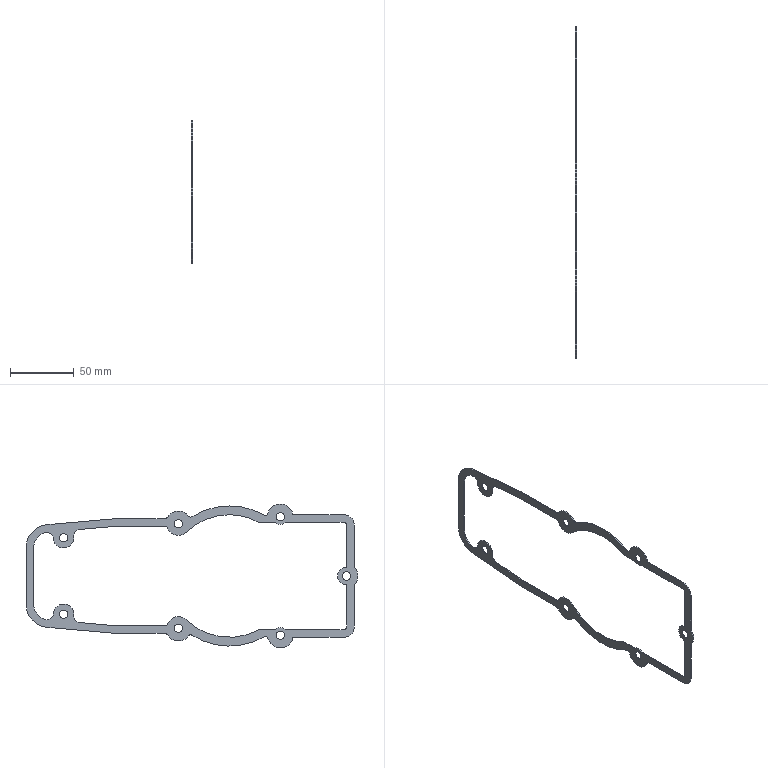Part | SolidWorks | features BaseBody 1 | 1 solid | 80 faces | box 0.8 x 260.5 x 113 mm | volume 3957 mm3 | cylinder 58 | plane 22 | commonest cylinder face diameters 6.5 x14 4 x10 20 x6 10 x5 16 x5 12 x3